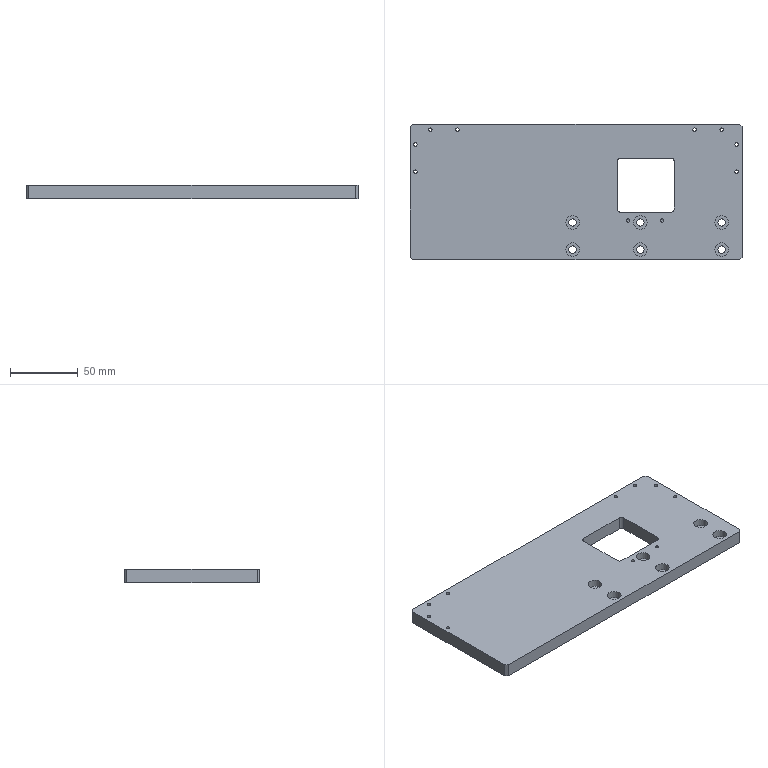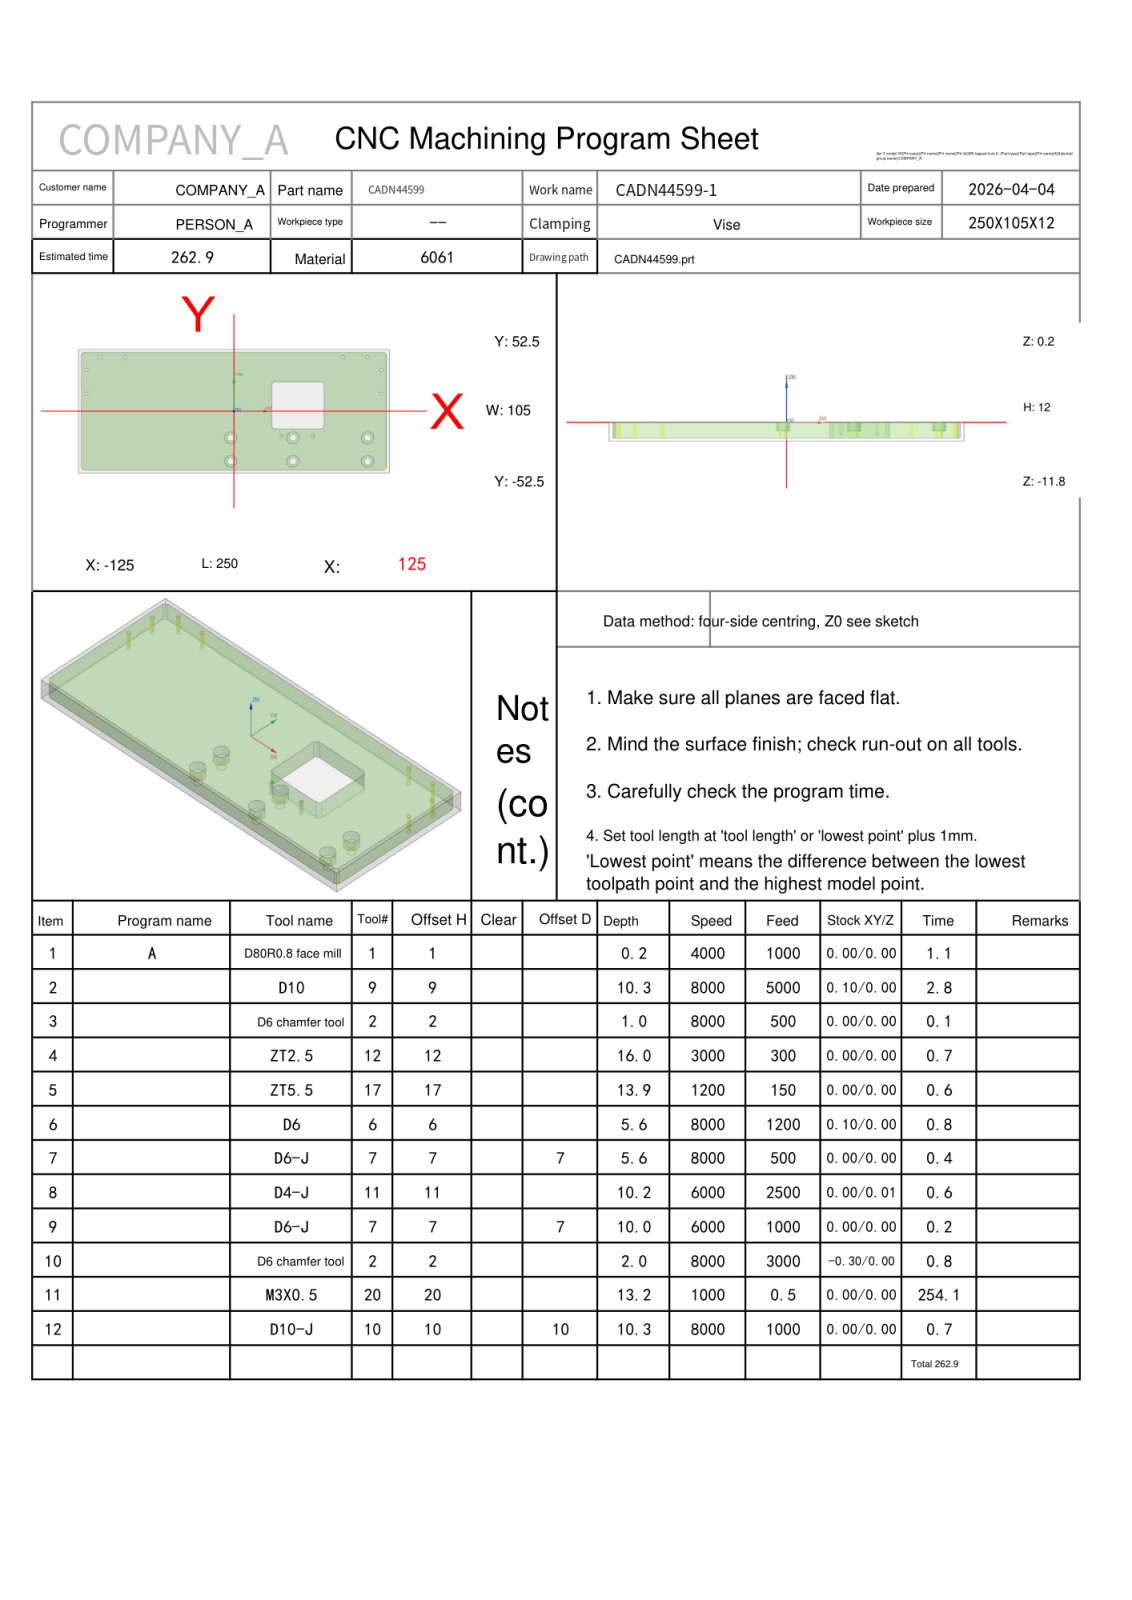NC program | NX | posted by the shop | part box 245 x 100 x 10 mm
Lines 1 to 754 of 5259:
%
O0001
(Machine time: 499.31 MIN)
(===Total Tool:10===)
(T1=D80R0.8 face mill D=80.  R=0.8  D-  H01 Z=0.    )
(T9=D10     D=10.  R=0.   D-  H09 Z=-10.1 )
(T2=D6 chamfer tool   D=6.   R=0.   D-  H02 Z=-1.75 )
(T12=ZT2.5  D=2.5  DR_a=118 D-  H12 Z=-15.75)
(T17=ZT5.5  D=5.5  DR_a=118 D-  H17 Z=-13.65)
(T6=D6      D=6.   R=0.   D-  H06 Z=-5.4  )
(T7=D6-J    D=6.   R=0.   D7  H07 Z=-9.8  )
(T11=D4-J   D=4.   R=0.   D-  H11 Z=-10.  )
(T20=M3X0.5 D=2.5  DR_a=180 D-  H20 Z=-13.  )
(T10=D10-J  D=10.  R=0.   D10 H10 Z=-10.1 )
G80 G90 G17 G49 G40
G91 G28 Z0
M01
N1 T01 M06
(D80R0.8 face mill  D=80. R=0.8 H=01 ce=0.00 di=0.00)
G00 G90 G54 X-167.5 Y45. M03 S4000
G43 H01 Z20.
M08
Z2.
G01 Z0.0 F1000.
X-162.5
X162.5
Y0.0
X-162.5
Y-45.
X162.5
X167.5
Z2.
G00 Z20.
G91 G28 Z0.0
M05
M09
G91 G28 Z0.0
M01
N2 T09 M06
(D10  D=10. R=0. H=09 ce=0.10 di=0.00)
G00 G90 G54 X0.0 Y55.1 M03 S8000
G43 H09 Z20.
M08
Z.5
G01 X120.5 Z.373 F5000.
G02 X124.106 Y53.606 Z.369 I0.0 J-5.1
G01 X126.106 Y51.606 Z.366
G02 X127.6 Y48. Z.361 I-3.606 J-3.606
G01 Y-48. Z.26
G02 X126.106 Y-51.606 Z.256 I-5.1 J0.0
G01 X124.106 Y-53.606 Z.253
G02 X122.515 Y-54.685 Z.251 I-3.606 J3.606
X120.5 Y-55.1 Z.249 I-2.015 J4.685
G01 X-120.5 Z-.006
G02 X-124.106 Y-53.606 Z-.01 I0.0 J5.1
G01 X-126.106 Y-51.606 Z-.013
G02 X-127.6 Y-48. Z-.017 I3.606 J3.606
G01 Y48. Z-.119
G02 X-126.106 Y51.606 Z-.123 I5.1 J0.0
G01 X-124.106 Y53.606 Z-.126
G02 X-120.5 Y55.1 Z-.13 I3.606 J-3.606
G01 X120.5 Z-.384
G02 X124.106 Y53.606 Z-.389 I0.0 J-5.1
G01 X126.106 Y51.606 Z-.392
G02 X127.6 Y48. Z-.396 I-3.606 J-3.606
G01 Y-48. Z-.497
G02 X126.106 Y-51.606 Z-.501 I-5.1 J0.0
G01 X124.106 Y-53.606 Z-.504
G02 X122.515 Y-54.685 Z-.506 I-3.606 J3.606
X120.5 Y-55.1 Z-.509 I-2.015 J4.685
G01 X-120.5 Z-.763
G02 X-124.106 Y-53.606 Z-.767 I0.0 J5.1
G01 X-126.106 Y-51.606 Z-.77
G02 X-127.6 Y-48. Z-.774 I3.606 J3.606
G01 Y48. Z-.876
G02 X-126.106 Y51.606 Z-.88 I5.1 J0.0
G01 X-124.106 Y53.606 Z-.883
G02 X-120.5 Y55.1 Z-.887 I3.606 J-3.606
G01 X120.5 Z-1.141
G02 X124.106 Y53.606 Z-1.146 I0.0 J-5.1
G01 X126.106 Y51.606 Z-1.149
G02 X127.6 Y48. Z-1.153 I-3.606 J-3.606
G01 Y-48. Z-1.254
G02 X126.106 Y-51.606 Z-1.258 I-5.1 J0.0
G01 X124.106 Y-53.606 Z-1.261
G02 X122.515 Y-54.685 Z-1.263 I-3.606 J3.606
X120.5 Y-55.1 Z-1.266 I-2.015 J4.685
G01 X-120.5 Z-1.52
G02 X-124.106 Y-53.606 Z-1.524 I0.0 J5.1
G01 X-126.106 Y-51.606 Z-1.527
G02 X-127.6 Y-48. Z-1.531 I3.606 J3.606
G01 Y48. Z-1.633
G02 X-126.106 Y51.606 Z-1.637 I5.1 J0.0
G01 X-124.106 Y53.606 Z-1.64
G02 X-120.5 Y55.1 Z-1.644 I3.606 J-3.606
G01 X120.5 Z-1.899
G02 X124.106 Y53.606 Z-1.903 I0.0 J-5.1
G01 X126.106 Y51.606 Z-1.906
G02 X127.6 Y48. Z-1.91 I-3.606 J-3.606
G01 Y-48. Z-2.011
G02 X126.106 Y-51.606 Z-2.016 I-5.1 J0.0
G01 X124.106 Y-53.606 Z-2.019
G02 X122.515 Y-54.685 Z-2.021 I-3.606 J3.606
X120.5 Y-55.1 Z-2.023 I-2.015 J4.685
G01 X-120.5 Z-2.277
G02 X-124.106 Y-53.606 Z-2.281 I0.0 J5.1
G01 X-126.106 Y-51.606 Z-2.284
G02 X-127.6 Y-48. Z-2.289 I3.606 J3.606
G01 Y48. Z-2.39
G02 X-126.106 Y51.606 Z-2.394 I5.1 J0.0
G01 X-124.106 Y53.606 Z-2.397
G02 X-120.5 Y55.1 Z-2.401 I3.606 J-3.606
G01 X120.5 Z-2.656
G02 X124.106 Y53.606 Z-2.66 I0.0 J-5.1
G01 X126.106 Y51.606 Z-2.663
G02 X127.6 Y48. Z-2.667 I-3.606 J-3.606
G01 Y-48. Z-2.769
G02 X126.106 Y-51.606 Z-2.773 I-5.1 J0.0
G01 X124.106 Y-53.606 Z-2.776
G02 X122.515 Y-54.685 Z-2.778 I-3.606 J3.606
X120.5 Y-55.1 Z-2.78 I-2.015 J4.685
G01 X-120.5 Z-3.034
G02 X-124.106 Y-53.606 Z-3.039 I0.0 J5.1
G01 X-126.106 Y-51.606 Z-3.042
G02 X-127.6 Y-48. Z-3.046 I3.606 J3.606
G01 Y48. Z-3.147
G02 X-126.106 Y51.606 Z-3.151 I5.1 J0.0
G01 X-124.106 Y53.606 Z-3.154
G02 X-120.5 Y55.1 Z-3.159 I3.606 J-3.606
G01 X120.5 Z-3.413
G02 X124.106 Y53.606 Z-3.417 I0.0 J-5.1
G01 X126.106 Y51.606 Z-3.42
G02 X127.6 Y48. Z-3.424 I-3.606 J-3.606
G01 Y-48. Z-3.526
G02 X126.106 Y-51.606 Z-3.53 I-5.1 J0.0
G01 X124.106 Y-53.606 Z-3.533
G02 X122.515 Y-54.685 Z-3.535 I-3.606 J3.606
X120.5 Y-55.1 Z-3.537 I-2.015 J4.685
G01 X-120.5 Z-3.791
G02 X-124.106 Y-53.606 Z-3.796 I0.0 J5.1
G01 X-126.106 Y-51.606 Z-3.799
G02 X-127.6 Y-48. Z-3.803 I3.606 J3.606
G01 Y48. Z-3.904
G02 X-126.106 Y51.606 Z-3.908 I5.1 J0.0
G01 X-124.106 Y53.606 Z-3.911
G02 X-120.5 Y55.1 Z-3.916 I3.606 J-3.606
G01 X120.5 Z-4.17
G02 X124.106 Y53.606 Z-4.174 I0.0 J-5.1
G01 X126.106 Y51.606 Z-4.177
G02 X127.6 Y48. Z-4.181 I-3.606 J-3.606
G01 Y-48. Z-4.283
G02 X126.106 Y-51.606 Z-4.287 I-5.1 J0.0
G01 X124.106 Y-53.606 Z-4.29
G02 X122.515 Y-54.685 Z-4.292 I-3.606 J3.606
X120.5 Y-55.1 Z-4.294 I-2.015 J4.685
G01 X-120.5 Z-4.549
G02 X-124.106 Y-53.606 Z-4.553 I0.0 J5.1
G01 X-126.106 Y-51.606 Z-4.556
G02 X-127.6 Y-48. Z-4.56 I3.606 J3.606
G01 Y48. Z-4.661
G02 X-126.106 Y51.606 Z-4.666 I5.1 J0.0
G01 X-124.106 Y53.606 Z-4.669
G02 X-120.5 Y55.1 Z-4.673 I3.606 J-3.606
G01 X120.5 Z-4.927
G02 X124.106 Y53.606 Z-4.931 I0.0 J-5.1
G01 X126.106 Y51.606 Z-4.934
G02 X127.6 Y48. Z-4.939 I-3.606 J-3.606
G01 Y-48. Z-5.04
G02 X126.106 Y-51.606 Z-5.044 I-5.1 J0.0
G01 X124.106 Y-53.606 Z-5.047
G02 X122.515 Y-54.685 Z-5.049 I-3.606 J3.606
X120.5 Y-55.1 Z-5.051 I-2.015 J4.685
G01 X-120.5 Z-5.306
G02 X-124.106 Y-53.606 Z-5.31 I0.0 J5.1
G01 X-126.106 Y-51.606 Z-5.313
G02 X-127.6 Y-48. Z-5.317 I3.606 J3.606
G01 Y48. Z-5.419
G02 X-126.106 Y51.606 Z-5.423 I5.1 J0.0
G01 X-124.106 Y53.606 Z-5.426
G02 X-120.5 Y55.1 Z-5.43 I3.606 J-3.606
G01 X120.5 Z-5.684
G02 X124.106 Y53.606 Z-5.689 I0.0 J-5.1
G01 X126.106 Y51.606 Z-5.692
G02 X127.6 Y48. Z-5.696 I-3.606 J-3.606
G01 Y-48. Z-5.797
G02 X126.106 Y-51.606 Z-5.801 I-5.1 J0.0
G01 X124.106 Y-53.606 Z-5.804
G02 X122.515 Y-54.685 Z-5.806 I-3.606 J3.606
X120.5 Y-55.1 Z-5.809 I-2.015 J4.685
G01 X-120.5 Z-6.063
G02 X-124.106 Y-53.606 Z-6.067 I0.0 J5.1
G01 X-126.106 Y-51.606 Z-6.07
G02 X-127.6 Y-48. Z-6.074 I3.606 J3.606
G01 Y48. Z-6.176
G02 X-126.106 Y51.606 Z-6.18 I5.1 J0.0
G01 X-124.106 Y53.606 Z-6.183
G02 X-120.5 Y55.1 Z-6.187 I3.606 J-3.606
G01 X120.5 Z-6.441
G02 X124.106 Y53.606 Z-6.446 I0.0 J-5.1
G01 X126.106 Y51.606 Z-6.449
G02 X127.6 Y48. Z-6.453 I-3.606 J-3.606
G01 Y-48. Z-6.554
G02 X126.106 Y-51.606 Z-6.558 I-5.1 J0.0
G01 X124.106 Y-53.606 Z-6.561
G02 X122.515 Y-54.685 Z-6.563 I-3.606 J3.606
X120.5 Y-55.1 Z-6.566 I-2.015 J4.685
G01 X-120.5 Z-6.82
G02 X-124.106 Y-53.606 Z-6.824 I0.0 J5.1
G01 X-126.106 Y-51.606 Z-6.827
G02 X-127.6 Y-48. Z-6.831 I3.606 J3.606
G01 Y48. Z-6.933
G02 X-126.106 Y51.606 Z-6.937 I5.1 J0.0
G01 X-124.106 Y53.606 Z-6.94
G02 X-120.5 Y55.1 Z-6.944 I3.606 J-3.606
G01 X120.5 Z-7.199
G02 X124.106 Y53.606 Z-7.203 I0.0 J-5.1
G01 X126.106 Y51.606 Z-7.206
G02 X127.6 Y48. Z-7.21 I-3.606 J-3.606
G01 Y-48. Z-7.311
G02 X126.106 Y-51.606 Z-7.316 I-5.1 J0.0
G01 X124.106 Y-53.606 Z-7.319
G02 X122.515 Y-54.685 Z-7.321 I-3.606 J3.606
X120.5 Y-55.1 Z-7.323 I-2.015 J4.685
G01 X-120.5 Z-7.577
G02 X-124.106 Y-53.606 Z-7.581 I0.0 J5.1
G01 X-126.106 Y-51.606 Z-7.584
G02 X-127.6 Y-48. Z-7.589 I3.606 J3.606
G01 Y48. Z-7.69
G02 X-126.106 Y51.606 Z-7.694 I5.1 J0.0
G01 X-124.106 Y53.606 Z-7.697
G02 X-120.5 Y55.1 Z-7.701 I3.606 J-3.606
G01 X120.5 Z-7.956
G02 X124.106 Y53.606 Z-7.96 I0.0 J-5.1
G01 X126.106 Y51.606 Z-7.963
G02 X127.6 Y48. Z-7.967 I-3.606 J-3.606
G01 Y-48. Z-8.069
G02 X126.106 Y-51.606 Z-8.073 I-5.1 J0.0
G01 X124.106 Y-53.606 Z-8.076
G02 X122.515 Y-54.685 Z-8.078 I-3.606 J3.606
X120.5 Y-55.1 Z-8.08 I-2.015 J4.685
G01 X-120.5 Z-8.334
G02 X-124.106 Y-53.606 Z-8.339 I0.0 J5.1
G01 X-126.106 Y-51.606 Z-8.342
G02 X-127.6 Y-48. Z-8.346 I3.606 J3.606
G01 Y48. Z-8.447
G02 X-126.106 Y51.606 Z-8.451 I5.1 J0.0
G01 X-124.106 Y53.606 Z-8.454
G02 X-120.5 Y55.1 Z-8.459 I3.606 J-3.606
G01 X120.5 Z-8.713
G02 X124.106 Y53.606 Z-8.717 I0.0 J-5.1
G01 X126.106 Y51.606 Z-8.72
G02 X127.6 Y48. Z-8.724 I-3.606 J-3.606
G01 Y-48. Z-8.826
G02 X126.106 Y-51.606 Z-8.83 I-5.1 J0.0
G01 X124.106 Y-53.606 Z-8.833
G02 X122.515 Y-54.685 Z-8.835 I-3.606 J3.606
X120.5 Y-55.1 Z-8.837 I-2.015 J4.685
G01 X-120.5 Z-9.091
G02 X-124.106 Y-53.606 Z-9.096 I0.0 J5.1
G01 X-126.106 Y-51.606 Z-9.099
G02 X-127.6 Y-48. Z-9.103 I3.606 J3.606
G01 Y48. Z-9.204
G02 X-126.106 Y51.606 Z-9.208 I5.1 J0.0
G01 X-124.106 Y53.606 Z-9.211
G02 X-120.5 Y55.1 Z-9.216 I3.606 J-3.606
G01 X120.5 Z-9.47
G02 X124.106 Y53.606 Z-9.474 I0.0 J-5.1
G01 X126.106 Y51.606 Z-9.477
G02 X127.6 Y48. Z-9.481 I-3.606 J-3.606
G01 Y-48. Z-9.583
G02 X126.106 Y-51.606 Z-9.587 I-5.1 J0.0
G01 X124.106 Y-53.606 Z-9.59
G02 X122.515 Y-54.685 Z-9.592 I-3.606 J3.606
X120.5 Y-55.1 Z-9.594 I-2.015 J4.685
G01 X-120.5 Z-9.849
G02 X-124.106 Y-53.606 Z-9.853 I0.0 J5.1
G01 X-126.106 Y-51.606 Z-9.856
G02 X-127.6 Y-48. Z-9.86 I3.606 J3.606
G01 Y48. Z-9.961
G02 X-126.106 Y51.606 Z-9.966 I5.1 J0.0
G01 X-124.106 Y53.606 Z-9.969
G02 X-120.5 Y55.1 Z-9.973 I3.606 J-3.606
G01 X0.0 Z-10.1
X120.5
G02 X124.106 Y53.606 I0.0 J-5.1
G01 X126.106 Y51.606
G02 X127.6 Y48. I-3.606 J-3.606
G01 Y-48.
G02 X126.106 Y-51.606 I-5.1 J0.0
G01 X124.106 Y-53.606
G02 X120.5 Y-55.1 I-3.606 J3.606
G01 X-120.5
G02 X-124.106 Y-53.606 I0.0 J5.1
G01 X-126.106 Y-51.606
G02 X-127.6 Y-48. I3.606 J3.606
G01 Y48.
G02 X-126.106 Y51.606 I5.1 J0.0
G01 X-124.106 Y53.606
G02 X-120.5 Y55.1 I3.606 J-3.606
G01 X0.0
X.5
Z-9.1
G00 Z20.
G00 G90 X51.5 Y19.9 M03 S6000
Z20.
Z.5
G01 X35.6 Z.437 F4000.
Y-9.9 Z.318
X67.4 Z.191
Y19.9 Z.073
X35.6 Z-.054
Y-9.9 Z-.172
X67.4 Z-.299
Y19.9 Z-.418
X35.6 Z-.544
Y-9.9 Z-.663
X67.4 Z-.789
Y19.9 Z-.908
X35.6 Z-1.035
Y-9.9 Z-1.153
X67.4 Z-1.28
Y19.9 Z-1.399
X35.6 Z-1.525
Y-9.9 Z-1.644
X67.4 Z-1.77
Y19.9 Z-1.889
X35.6 Z-2.016
Y-9.9 Z-2.134
X67.4 Z-2.261
Y19.9 Z-2.38
X35.6 Z-2.506
Y-9.9 Z-2.625
X67.4 Z-2.751
Y19.9 Z-2.87
X35.6 Z-2.997
Y-9.9 Z-3.115
X67.4 Z-3.242
Y19.9 Z-3.361
X35.6 Z-3.487
Y-9.9 Z-3.606
X67.4 Z-3.732
Y19.9 Z-3.851
X35.6 Z-3.978
Y-9.9 Z-4.096
X67.4 Z-4.223
Y19.9 Z-4.341
X35.6 Z-4.468
Y-9.9 Z-4.587
X67.4 Z-4.713
Y19.9 Z-4.832
X35.6 Z-4.959
Y-9.9 Z-5.077
X67.4 Z-5.204
Y19.9 Z-5.322
X35.6 Z-5.449
Y-9.9 Z-5.568
X67.4 Z-5.694
Y19.9 Z-5.813
X35.6 Z-5.939
Y-9.9 Z-6.058
X67.4 Z-6.185
Y19.9 Z-6.303
X35.6 Z-6.43
Y-9.9 Z-6.549
X67.4 Z-6.675
Y19.9 Z-6.794
X35.6 Z-6.92
Y-9.9 Z-7.039
X67.4 Z-7.166
Y19.9 Z-7.284
X35.6 Z-7.411
Y-9.9 Z-7.53
X67.4 Z-7.656
Y19.9 Z-7.775
X35.6 Z-7.901
Y-9.9 Z-8.02
X67.4 Z-8.147
Y19.9 Z-8.265
X35.6 Z-8.392
Y-9.9 Z-8.511
X67.4 Z-8.637
Y19.9 Z-8.756
X35.6 Z-8.882
Y-9.9 Z-9.001
X67.4 Z-9.128
Y19.9 Z-9.246
X35.6 Z-9.373
Y-9.9 Z-9.491
X67.4 Z-9.618
Y19.9 Z-9.737
X51.5 Z-9.8
X35.6
Y-9.9
X67.4
Y19.9
X51.5
X51.
Z-8.8
G00 Z20.
G91 G28 Z0.0
M05
M09
G91 G28 Z0.0
M01
N3 T02 M06
(D6 chamfer tool  D=6. R=0. H=02 ce=0.00 di=0.00)
G00 G90 G54 X-118.5 Y15. M03 S8000
G43 H02 Z20.
M08
G98 G81 X-118.5 Y15. Z-.8 R1. F500.
Y35.
X-107.5 Y46.
X-87.5
X-2.5 Y-22.5
Y-42.5
X47.5
X38.5 Y-21.
X47.5 Y-22.5
X63.5 Y-21.
X107.5 Y-42.5
Y-22.5
X118.5 Y15.
Y35.
X107.5 Y46.
X87.5
G80
G00 Z20.
G91 G28 Z0.0
M05
M09
G91 G28 Z0.0
M01
N4 T12 M06
(ZT2.5 D=2.5 DR_a=118 H=12)
G00 G90 G54 X118.5 Y15. M03 S3000
G43 H12 Z20.
M08
G98 G83 X118.5 Y15. Z-15.751 R1. F300. Q2.
Y35.
X107.5 Y46.
X87.5
X-87.5
X-107.5
X-118.5 Y35.
Y15.
G80
G00 Z20.
G00 G90 X38.5 Y-21. M03 S3000
Z20.
G98 G83 X38.5 Y-21. Z-9. R1. F100. Q2.
X63.5
G80
G00 Z20.
G91 G28 Z0.0
M05
M09
G91 G28 Z0.0
M01
N5 T17 M06
(ZT5.5 D=5.5 DR_a=118 H=17)
G00 G90 G54 X107.5 Y-22.5 M03 S1200
G43 H17 Z20.
M08
G98 G83 X107.5 Y-22.5 Z-13.652 R1. F150. Q2.
Y-42.5
X47.5
Y-22.5
X-2.5
Y-42.5
G80
G00 Z20.
G91 G28 Z0.0
M05
M09
G91 G28 Z0.0
M01
N6 T06 M06
(D6  D=6. R=0. H=06 ce=0.10 di=0.00)
G00 G90 G54 X107.5 Y-22.5 M03 S8000
G43 H06 Z20.
M08
Z.5
G03 X108.45 Y-23.45 I.95 J0.0 F1200.
X109.4 Y-22.5 I0.0 J.95
X109.4 Y-22.5 Z0.0 I-1.9 J0.0
X109.4 Y-22.5 Z-.5 I-1.9 J0.0
X109.4 Y-22.5 Z-1. I-1.9 J0.0
X109.4 Y-22.5 Z-1.5 I-1.9 J0.0
X109.4 Y-22.5 Z-2. I-1.9 J0.0
X109.4 Y-22.5 Z-2.5 I-1.9 J0.0
X109.4 Y-22.5 Z-3. I-1.9 J0.0
X109.4 Y-22.5 Z-3.5 I-1.9 J0.0
X109.4 Y-22.5 Z-4. I-1.9 J0.0
X109.4 Y-22.5 Z-4.5 I-1.9 J0.0
X109.4 Y-22.5 Z-5. I-1.9 J0.0
X108.087 Y-24.307 Z-5.4 I-1.9 J0.0
X109.4 Y-22.5 I-.587 J1.807
X107.5 Y-20.6 I-1.9 J0.0
X105.6 Y-22.5 I0.0 J-1.9
X107.5 Y-24.4 I1.9 J0.0
X108.087 Y-24.307 I0.0 J1.9
X108.744 Y-23.404 I-.294 J.904
X107.794 Y-22.454 I-.95 J0.0
X107.5 Y-22.5 I0.0 J-.95
G00 Z20.
Y-42.5
Z.5
G03 X108.45 Y-43.45 I.95 J0.0
X109.4 Y-42.5 I0.0 J.95
X109.4 Y-42.5 Z0.0 I-1.9 J0.0
X109.4 Y-42.5 Z-.5 I-1.9 J0.0
X109.4 Y-42.5 Z-1. I-1.9 J0.0
X109.4 Y-42.5 Z-1.5 I-1.9 J0.0
X109.4 Y-42.5 Z-2. I-1.9 J0.0
X109.4 Y-42.5 Z-2.5 I-1.9 J0.0
X109.4 Y-42.5 Z-3. I-1.9 J0.0
X109.4 Y-42.5 Z-3.5 I-1.9 J0.0
X109.4 Y-42.5 Z-4. I-1.9 J0.0
X109.4 Y-42.5 Z-4.5 I-1.9 J0.0
X109.4 Y-42.5 Z-5. I-1.9 J0.0
X108.087 Y-44.307 Z-5.4 I-1.9 J0.0
X109.4 Y-42.5 I-.587 J1.807
X107.5 Y-40.6 I-1.9 J0.0
X105.6 Y-42.5 I0.0 J-1.9
X107.5 Y-44.4 I1.9 J0.0
X108.087 Y-44.307 I0.0 J1.9
X108.744 Y-43.404 I-.294 J.904
X107.794 Y-42.454 I-.95 J0.0
X107.5 Y-42.5 I0.0 J-.95
G00 Z20.
X47.5
Z.5
G03 X48.45 Y-43.45 I.95 J0.0
X49.4 Y-42.5 I0.0 J.95
X49.4 Y-42.5 Z0.0 I-1.9 J0.0
X49.4 Y-42.5 Z-.5 I-1.9 J0.0
X49.4 Y-42.5 Z-1. I-1.9 J0.0
X49.4 Y-42.5 Z-1.5 I-1.9 J0.0
X49.4 Y-42.5 Z-2. I-1.9 J0.0
X49.4 Y-42.5 Z-2.5 I-1.9 J0.0
X49.4 Y-42.5 Z-3. I-1.9 J0.0
X49.4 Y-42.5 Z-3.5 I-1.9 J0.0
X49.4 Y-42.5 Z-4. I-1.9 J0.0
X49.4 Y-42.5 Z-4.5 I-1.9 J0.0
X49.4 Y-42.5 Z-5. I-1.9 J0.0
X48.087 Y-44.307 Z-5.4 I-1.9 J0.0
X49.4 Y-42.5 I-.587 J1.807
X47.5 Y-40.6 I-1.9 J0.0
X45.6 Y-42.5 I0.0 J-1.9
X47.5 Y-44.4 I1.9 J0.0
X48.087 Y-44.307 I0.0 J1.9
X48.744 Y-43.404 I-.294 J.904
X47.794 Y-42.454 I-.95 J0.0
X47.5 Y-42.5 I0.0 J-.95
G00 Z20.
Y-22.5
Z.5
G03 X48.45 Y-23.45 I.95 J0.0
X49.4 Y-22.5 I0.0 J.95
X49.4 Y-22.5 Z0.0 I-1.9 J0.0
X49.4 Y-22.5 Z-.5 I-1.9 J0.0
X49.4 Y-22.5 Z-1. I-1.9 J0.0
X49.4 Y-22.5 Z-1.5 I-1.9 J0.0
X49.4 Y-22.5 Z-2. I-1.9 J0.0
X49.4 Y-22.5 Z-2.5 I-1.9 J0.0
X49.4 Y-22.5 Z-3. I-1.9 J0.0
X49.4 Y-22.5 Z-3.5 I-1.9 J0.0
X49.4 Y-22.5 Z-4. I-1.9 J0.0
X49.4 Y-22.5 Z-4.5 I-1.9 J0.0
X49.4 Y-22.5 Z-5. I-1.9 J0.0
X48.087 Y-24.307 Z-5.4 I-1.9 J0.0
X49.4 Y-22.5 I-.587 J1.807
X47.5 Y-20.6 I-1.9 J0.0
X45.6 Y-22.5 I0.0 J-1.9
X47.5 Y-24.4 I1.9 J0.0
X48.087 Y-24.307 I0.0 J1.9
X48.744 Y-23.404 I-.294 J.904
X47.794 Y-22.454 I-.95 J0.0
X47.5 Y-22.5 I0.0 J-.95
G00 Z20.
X-2.5
Z.5
G03 X-1.55 Y-23.45 I.95 J0.0
X-.6 Y-22.5 I0.0 J.95
X-.6 Y-22.5 Z0.0 I-1.9 J0.0
X-.6 Y-22.5 Z-.5 I-1.9 J0.0
X-.6 Y-22.5 Z-1. I-1.9 J0.0
X-.6 Y-22.5 Z-1.5 I-1.9 J0.0
X-.6 Y-22.5 Z-2. I-1.9 J0.0
X-.6 Y-22.5 Z-2.5 I-1.9 J0.0
X-.6 Y-22.5 Z-3. I-1.9 J0.0
X-.6 Y-22.5 Z-3.5 I-1.9 J0.0
X-.6 Y-22.5 Z-4. I-1.9 J0.0
X-.6 Y-22.5 Z-4.5 I-1.9 J0.0
X-.6 Y-22.5 Z-5. I-1.9 J0.0
X-1.913 Y-24.307 Z-5.4 I-1.9 J0.0
X-.6 Y-22.5 I-.587 J1.807
X-2.5 Y-20.6 I-1.9 J0.0
X-4.4 Y-22.5 I0.0 J-1.9
X-2.5 Y-24.4 I1.9 J0.0
X-1.913 Y-24.307 I0.0 J1.9
X-1.256 Y-23.404 I-.294 J.904
X-2.206 Y-22.454 I-.95 J0.0
X-2.5 Y-22.5 I0.0 J-.95
G00 Z20.
Y-42.5
Z.5
G03 X-1.55 Y-43.45 I.95 J0.0
X-.6 Y-42.5 I0.0 J.95
X-.6 Y-42.5 Z0.0 I-1.9 J0.0
X-.6 Y-42.5 Z-.5 I-1.9 J0.0
X-.6 Y-42.5 Z-1. I-1.9 J0.0
X-.6 Y-42.5 Z-1.5 I-1.9 J0.0
X-.6 Y-42.5 Z-2. I-1.9 J0.0
X-.6 Y-42.5 Z-2.5 I-1.9 J0.0
X-.6 Y-42.5 Z-3. I-1.9 J0.0
X-.6 Y-42.5 Z-3.5 I-1.9 J0.0
X-.6 Y-42.5 Z-4. I-1.9 J0.0
X-.6 Y-42.5 Z-4.5 I-1.9 J0.0
X-.6 Y-42.5 Z-5. I-1.9 J0.0
X-1.913 Y-44.307 Z-5.4 I-1.9 J0.0
X-.6 Y-42.5 I-.587 J1.807
X-2.5 Y-40.6 I-1.9 J0.0
X-4.4 Y-42.5 I0.0 J-1.9
X-2.5 Y-44.4 I1.9 J0.0
X-1.913 Y-44.307 I0.0 J1.9
X-1.256 Y-43.404 I-.294 J.904
X-2.206 Y-42.454 I-.95 J0.0
X-2.5 Y-42.5 I0.0 J-.95
G00 Z20.
G91 G28 Z0.0
M05
M09
G91 G28 Z0.0
M01
N7 T07 M06
(D6-J  D=6. R=0. H=07 ce=0.00 di=0.00)
G00 G90 G54 X107.5 Y-22.5 M03 S8000
G43 H07 Z20.
M08
Z0.0
G41 D07
G01 X107.54 Y-22.696 F500.
G03 X108.51 Y-23.49 I.97 J.196
X109.5 Y-22.5 I0.0 J.99
X109.5 Y-22.5 Z-5. I-2. J0.0
X109.253 Y-21.536 Z-5.4 I-2. J0.0
X107.5 Y-20.5 I-1.753 J-.964
X105.5 Y-22.5 I0.0 J-2.
X107.5 Y-24.5 I2. J0.0
X109.5 Y-22.5 I0.0 J2.
X109.253 Y-21.536 I-2. J0.0
X108.385 Y-21.023 I-.868 J-.477
X107.395 Y-22.013 I0.0 J-.99
X107.44 Y-22.309 I.99 J0.0
G01 G40 X107.5 Y-22.5
G00 Z20.
Y-42.5
Z0.0
G41 D07
G01 X107.54 Y-42.696
G03 X108.51 Y-43.49 I.97 J.196
X109.5 Y-42.5 I0.0 J.99
X109.5 Y-42.5 Z-5. I-2. J0.0
X109.253 Y-41.536 Z-5.4 I-2. J0.0
X107.5 Y-40.5 I-1.753 J-.964
X105.5 Y-42.5 I0.0 J-2.
X107.5 Y-44.5 I2. J0.0
X109.5 Y-42.5 I0.0 J2.
X109.253 Y-41.536 I-2. J0.0
X108.385 Y-41.023 I-.868 J-.477
X107.395 Y-42.013 I0.0 J-.99
X107.44 Y-42.309 I.99 J0.0
G01 G40 X107.5 Y-42.5
G00 Z20.
X47.5
Z0.0
G41 D07
G01 X47.54 Y-42.696
G03 X48.51 Y-43.49 I.97 J.196
X49.5 Y-42.5 I0.0 J.99
X49.5 Y-42.5 Z-5. I-2. J0.0
X49.253 Y-41.536 Z-5.4 I-2. J0.0
X47.5 Y-40.5 I-1.753 J-.964
X45.5 Y-42.5 I0.0 J-2.
X47.5 Y-44.5 I2. J0.0
X49.5 Y-42.5 I0.0 J2.
X49.253 Y-41.536 I-2. J0.0
X48.385 Y-41.023 I-.868 J-.477
X47.395 Y-42.013 I0.0 J-.99
X47.44 Y-42.309 I.99 J0.0
G01 G40 X47.5 Y-42.5
G00 Z20.
Y-22.5
Z0.0
G41 D07
G01 X47.54 Y-22.696
G03 X48.51 Y-23.49 I.97 J.196
X49.5 Y-22.5 I0.0 J.99
X49.5 Y-22.5 Z-5. I-2. J0.0
X49.253 Y-21.536 Z-5.4 I-2. J0.0
X47.5 Y-20.5 I-1.753 J-.964
X45.5 Y-22.5 I0.0 J-2.
X47.5 Y-24.5 I2. J0.0
X49.5 Y-22.5 I0.0 J2.
X49.253 Y-21.536 I-2. J0.0
X48.385 Y-21.023 I-.868 J-.477
X47.395 Y-22.013 I0.0 J-.99
X47.44 Y-22.309 I.99 J0.0
G01 G40 X47.5 Y-22.5
G00 Z20.
X-2.5
Z0.0
G41 D07
G01 X-2.46 Y-22.696
G03 X-1.49 Y-23.49 I.97 J.196
X-.5 Y-22.5 I0.0 J.99
X-.5 Y-22.5 Z-5. I-2. J0.0
X-.747 Y-21.536 Z-5.4 I-2. J0.0
X-2.5 Y-20.5 I-1.753 J-.964
X-4.5 Y-22.5 I0.0 J-2.
X-2.5 Y-24.5 I2. J0.0
X-.5 Y-22.5 I0.0 J2.
X-.747 Y-21.536 I-2. J0.0
X-1.615 Y-21.023 I-.868 J-.477
X-2.605 Y-22.013 I0.0 J-.99
X-2.56 Y-22.309 I.99 J0.0
G01 G40 X-2.5 Y-22.5
G00 Z20.
Y-42.5
Z0.0
G41 D07
G01 X-2.46 Y-42.696
G03 X-1.49 Y-43.49 I.97 J.196
X-.5 Y-42.5 I0.0 J.99
X-.5 Y-42.5 Z-5. I-2. J0.0
X-.747 Y-41.536 Z-5.4 I-2. J0.0
X-2.5 Y-40.5 I-1.753 J-.964
X-4.5 Y-42.5 I0.0 J-2.
X-2.5 Y-44.5 I2. J0.0
X-.5 Y-42.5 I0.0 J2.
X-.747 Y-41.536 I-2. J0.0
X-1.615 Y-41.023 I-.868 J-.477
X-2.605 Y-42.013 I0.0 J-.99
X-2.56 Y-42.309 I.99 J0.0
G01 G40 X-2.5 Y-42.5
G00 Z20.
G91 G28 Z0.0
M05
M09
G91 G28 Z0.0
M01